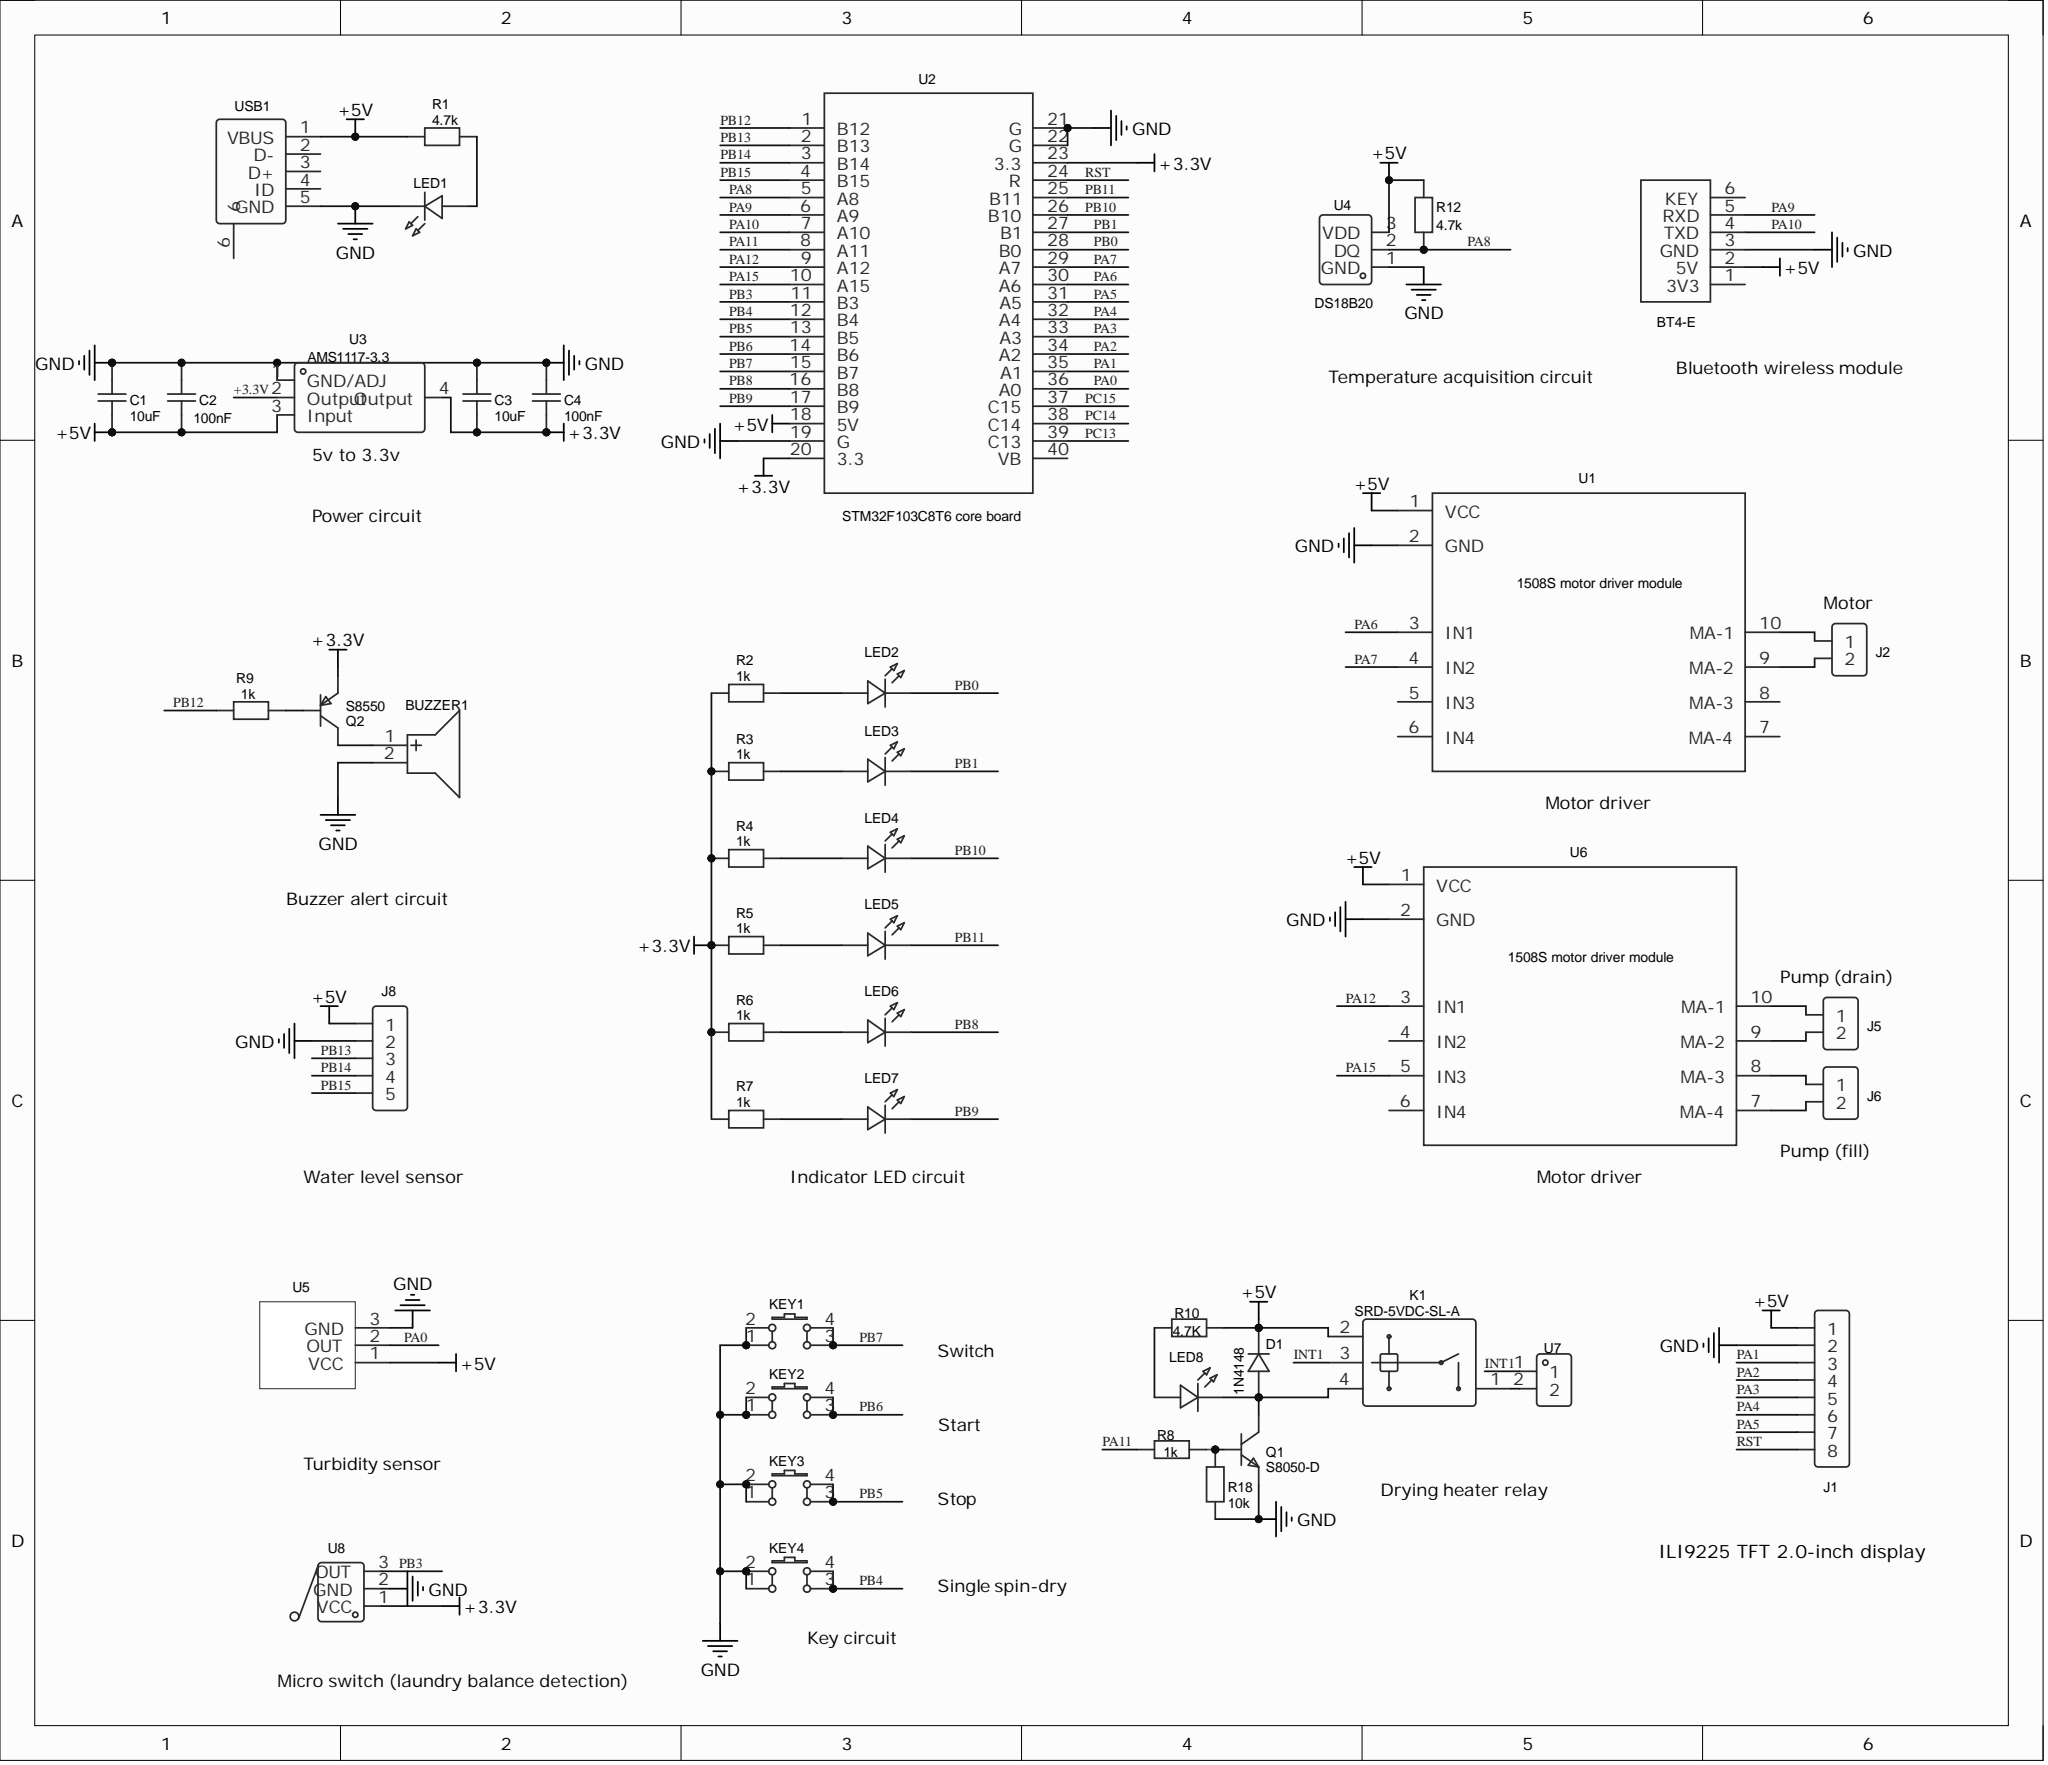Circuit board | Altium Designer | 48 parts | 53 nets
Bill of materials:
Comment,Description,Designator,Footprint,LibRef,Quantity
"NO","","BT4-E","HDR1X6","NO","1"
"5V","","BUZZER1","PIN2","5V","1"
"10uF","","C1, C3","C0805","10uF","2"
"100nF","","C2, C4","C0805","100nF","2"
"1N4148","","D1","DO-35","1N4148","1"
"HDR-M-2.54_1x8","","J1","HDR1X8","HDR-M-2.54_1x8","1"
"HDR-M-2.54_1x2","","J2, J5, J6","HDR1X2","HDR-M-2.54_1x2","3"
"HDR-M-2.54_1x5","","J8","HDR1X5","HDR-M-2.54_1x5","1"
"SRD-5VDC-SL-A","","K1","012-1HW_BK","SRD-5VDC-SL-A","1"
"K4-6×6_TH","","KEY1, KEY2, KEY3, KEY4","四脚轻触开关","K4-6×6_TH","4"
"LED-TH-3mm_R","","LED1, LED8","LED-1","LED-TH-3mm_R","2"
"LED-0603_R","","LED2, LED3, LED4, LED5, LED6, LED7","LED-1","LED-0603_R","6"
"S8050-D","","Q1","TO-92A","S8050-D","1"
"S8550","","Q2","TO-92A","S8550","1"
"4.7k","","R1, R10, R12","AXIAL-0.3","4.7k","3"
"1k","","R2, R3, R4, R5, R6, R7, R8, R9","AXIAL-0.3","1k","8"
"10k","","R18","AXIAL-0.3","10k","1"
"1508S motor driver module","","U1, U6","DIANJIQUDONG","电机驱动1508S模块","2"
"STM32F103C8T6 core board","","U2","STM32核心板","STM32F103C8T6核心板","1"
"AMS1117-3.3","","U3","AMS1117-3.3","AMS1117-3.3","1"
"DS18B20","","U4","DS18B20","DS18B20","1"
"NO","","U5","HDR1X3","NO","1"
"Connect watering pump","","U7","HDR1X2","接浇水水泵","1"
"NO","","U8","xianwei","NO","1"
"MICRO5.9MMUSB","","USB1","MICRO-USB-SMD_5P-P0.65-H-F_MICRO5.9MMUSB","MICRO5.9MMUSB","1"
Netlist (Protel format):
[
BT4-E
HDR1X6
NO



]
[
BUZZER1
PIN2
5V



]
[
C1
C0805
10uF



]
[
C2
C0805
100nF



]
[
C3
C0805
10uF



]
[
C4
C0805
100nF



]
[
D1
DO-35
1N4148



]
[
J1
HDR1X8
HDR-M-2.54_1x8



]
[
J2
HDR1X2
HDR-M-2.54_1x2



]
[
J5
HDR1X2
HDR-M-2.54_1x2



]
[
J6
HDR1X2
HDR-M-2.54_1x2



]
[
J8
HDR1X5
HDR-M-2.54_1x5



]
[
K1
012-1HW_BK
SRD-5VDC-SL-A



]
[
KEY1
四脚轻触开关
K4-6×6_TH



]
[
KEY2
四脚轻触开关
K4-6×6_TH



]
[
KEY3
四脚轻触开关
K4-6×6_TH



]
[
KEY4
四脚轻触开关
K4-6×6_TH



]
[
LED1
LED-1
LED-TH-3mm_R



]
[
LED2
LED-1
LED-0603_R



]
[
LED3
LED-1
LED-0603_R



]
[
LED4
LED-1
LED-0603_R



]
[
LED5
LED-1
LED-0603_R



]
[
LED6
LED-1
LED-0603_R



]
[
LED7
LED-1
LED-0603_R



]
[
LED8
LED-1
LED-TH-3mm_R



]
[
Q1
TO-92A
S8050-D



]
[
Q2
TO-92A
S8550



]
[
R1
AXIAL-0.3
4.7k



]
[
R2
AXIAL-0.3
1k



]
[
R3
AXIAL-0.3
1k



]
[
R4
AXIAL-0.3
1k



]
[
R5
AXIAL-0.3
1k



]
[
R6
AXIAL-0.3
1k



]
[
R7
AXIAL-0.3
1k



]
[
R8
AXIAL-0.3
1k



]
[
R9
AXIAL-0.3
1k



]
[
R10
AXIAL-0.3
4.7K



]
[
R12
AXIAL-0.3
4.7k



]
[
R18
AXIAL-0.3
10k



]
[
U1
DIANJIQUDONG
1508S motor driver module



]
[
U2
STM32核心板
STM32F103C8T6 core board



]
[
U3
AMS1117-3.3
AMS1117-3.3



]
[
U4
DS18B20
DS18B20



]
[
U5
HDR1X3
NO



]
[
U6
DIANJIQUDONG
1508S motor driver module



]
[
U7
HDR1X2
Connect watering pump



]
[
U8
xianwei
NO



]
[
USB1
MICRO-USB-SMD_5P-P0.65-H-F_MICRO5.9MMUSB
MICRO5.9MMUSB



]
(
RST
J1-8
U2-24
)
(
PB15
J8-5
U2-4
)
(
PB14
J8-4
U2-3
)
(
PB13
J8-3
U2-2
)
(
PB12
R9-1
U2-1
)
(
PB11
LED5-2
U2-25
)
(
PB10
LED4-2
U2-26
)
(
PB9
LED7-2
U2-17
)
(
PB8
LED6-2
U2-16
)
(
PB7
KEY1-3
KEY1-4
U2-15
)
(
PB6
KEY2-3
KEY2-4
U2-14
)
(
PB5
KEY3-3
KEY3-4
U2-13
)
(
PB4
KEY4-3
KEY4-4
U2-12
)
(
PB3
U2-11
U8-3
)
(
PB1
LED3-2
U2-27
)
(
PB0
LED2-2
U2-28
)
(
PA15
U2-10
U6-5
)
(
PA12
U2-9
U6-3
)
(
PA11
R8-1
U2-8
)
(
PA10
BT4-E-4
U2-7
)
(
PA9
BT4-E-5
U2-6
)
(
PA8
R12-1
U2-5
U4-2
)
(
PA7
U1-4
U2-29
)
(
PA6
U1-3
U2-30
)
(
PA5
J1-7
U2-31
)
(
PA4
J1-6
U2-32
)
(
PA3
J1-5
U2-33
)
(
PA2
J1-4
U2-34
)
(
PA1
J1-3
U2-35
)
(
PA0
U2-36
U5-2
)
(
NetQ2_2
Q2-2
R9-2
)
(
NetQ1_2
Q1-2
R8-2
R18-2
)
(
NetLED8_1
LED8-1
R10-1
)
(
NetLED7_1
LED7-1
R7-2
)
(
NetLED6_1
LED6-1
R6-2
)
(
NetLED5_1
LED5-1
R5-2
)
(
NetLED4_1
LED4-1
R4-2
)
(
NetLED3_1
LED3-1
R3-2
)
(
NetLED2_1
LED2-1
R2-2
)
(
NetLED1_1
LED1-1
R1-2
)
(
NetK1_1
K1-1
U7-2
)
(
NetJ6_2
J6-2
U6-7
)
(
NetJ6_1
J6-1
U6-8
)
(
NetJ5_2
J5-2
U6-9
)
(
NetJ5_1
J5-1
U6-10
)
(
NetJ2_2
J2-2
U1-9
)
(
NetJ2_1
J2-1
U1-10
)
(
NetD1_2
D1-2
K1-4
LED8-2
Q1-3
)
(
NetBUZZER1_1
BUZZER1-1
Q2-3
)
(
INT1
K1-3
U7-1
)
(
GND
BT4-E-3
BUZZER1-2
C1-2
C2-2
C3-1
C4-2
J1-2
J8-2
KEY1-1
KEY1-2
KEY2-1
KEY2-2
KEY3-1
KEY3-2
KEY4-1
KEY4-2
LED1-2
Q1-1
R18-1
U1-2
U2-19
U2-21
U2-22
U3-1
U4-1
U5-3
U6-2
U8-2
USB1-5
)
(
+5V
BT4-E-2
C1-1
C2-1
D1-1
J1-1
J8-1
K1-2
R1-1
R10-2
R12-2
U1-1
U2-18
U3-3
U4-3
U5-1
U6-1
USB1-1
)
(
+3.3V
C3-2
C4-1
Q2-1
R2-1
R3-1
R4-1
R5-1
R6-1
R7-1
U2-20
U2-23
U3-2
U3-4
U8-1
)